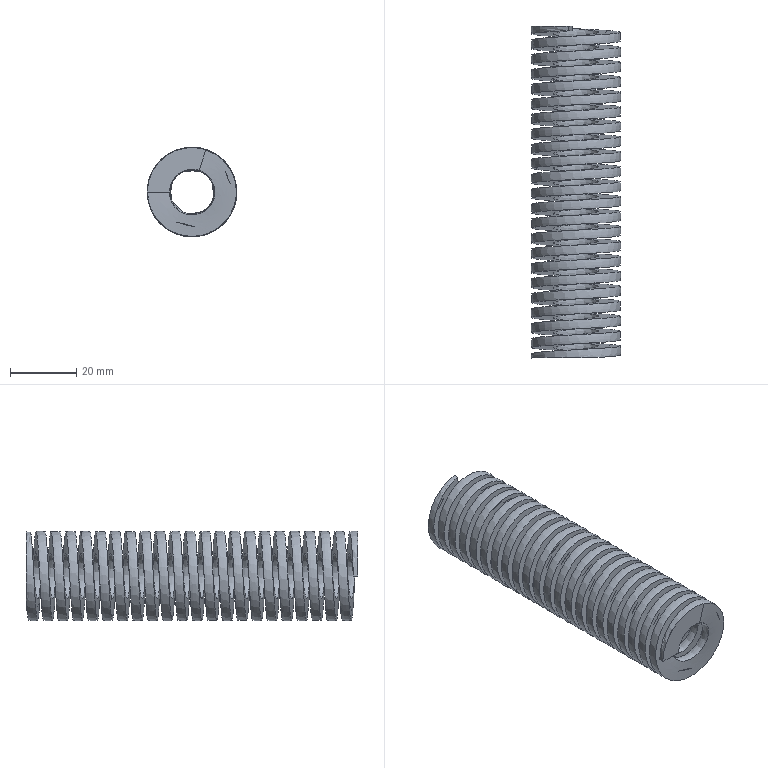Part | Creo | 1 solid | 8 faces | box 27.01 x 100 x 26.908 mm | volume 25635 mm3 | spline 4 | plane 4